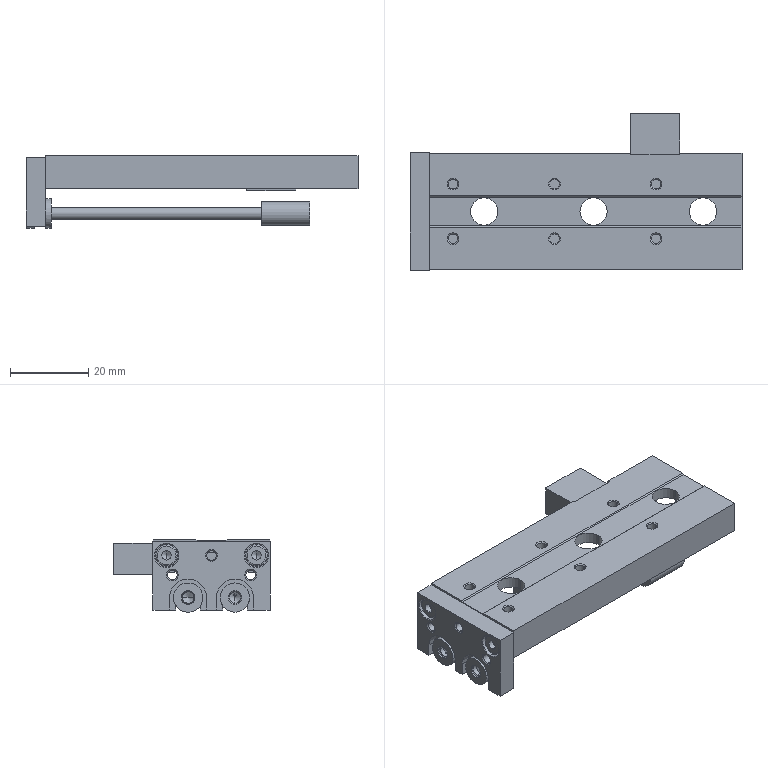Part | STEP file | 11-_HLQ6X40-S-A-0-rod11 | 1 solid | 230 faces | box 85 x 40 x 18.55 mm | volume 17833 mm3 | plane 88 | cylinder 84 | cone 50 | spline 8 | commonest cylinder face diameters 2.459 x22 5.5 x8 6 x8 7.5 x8 7 x6 2 x4